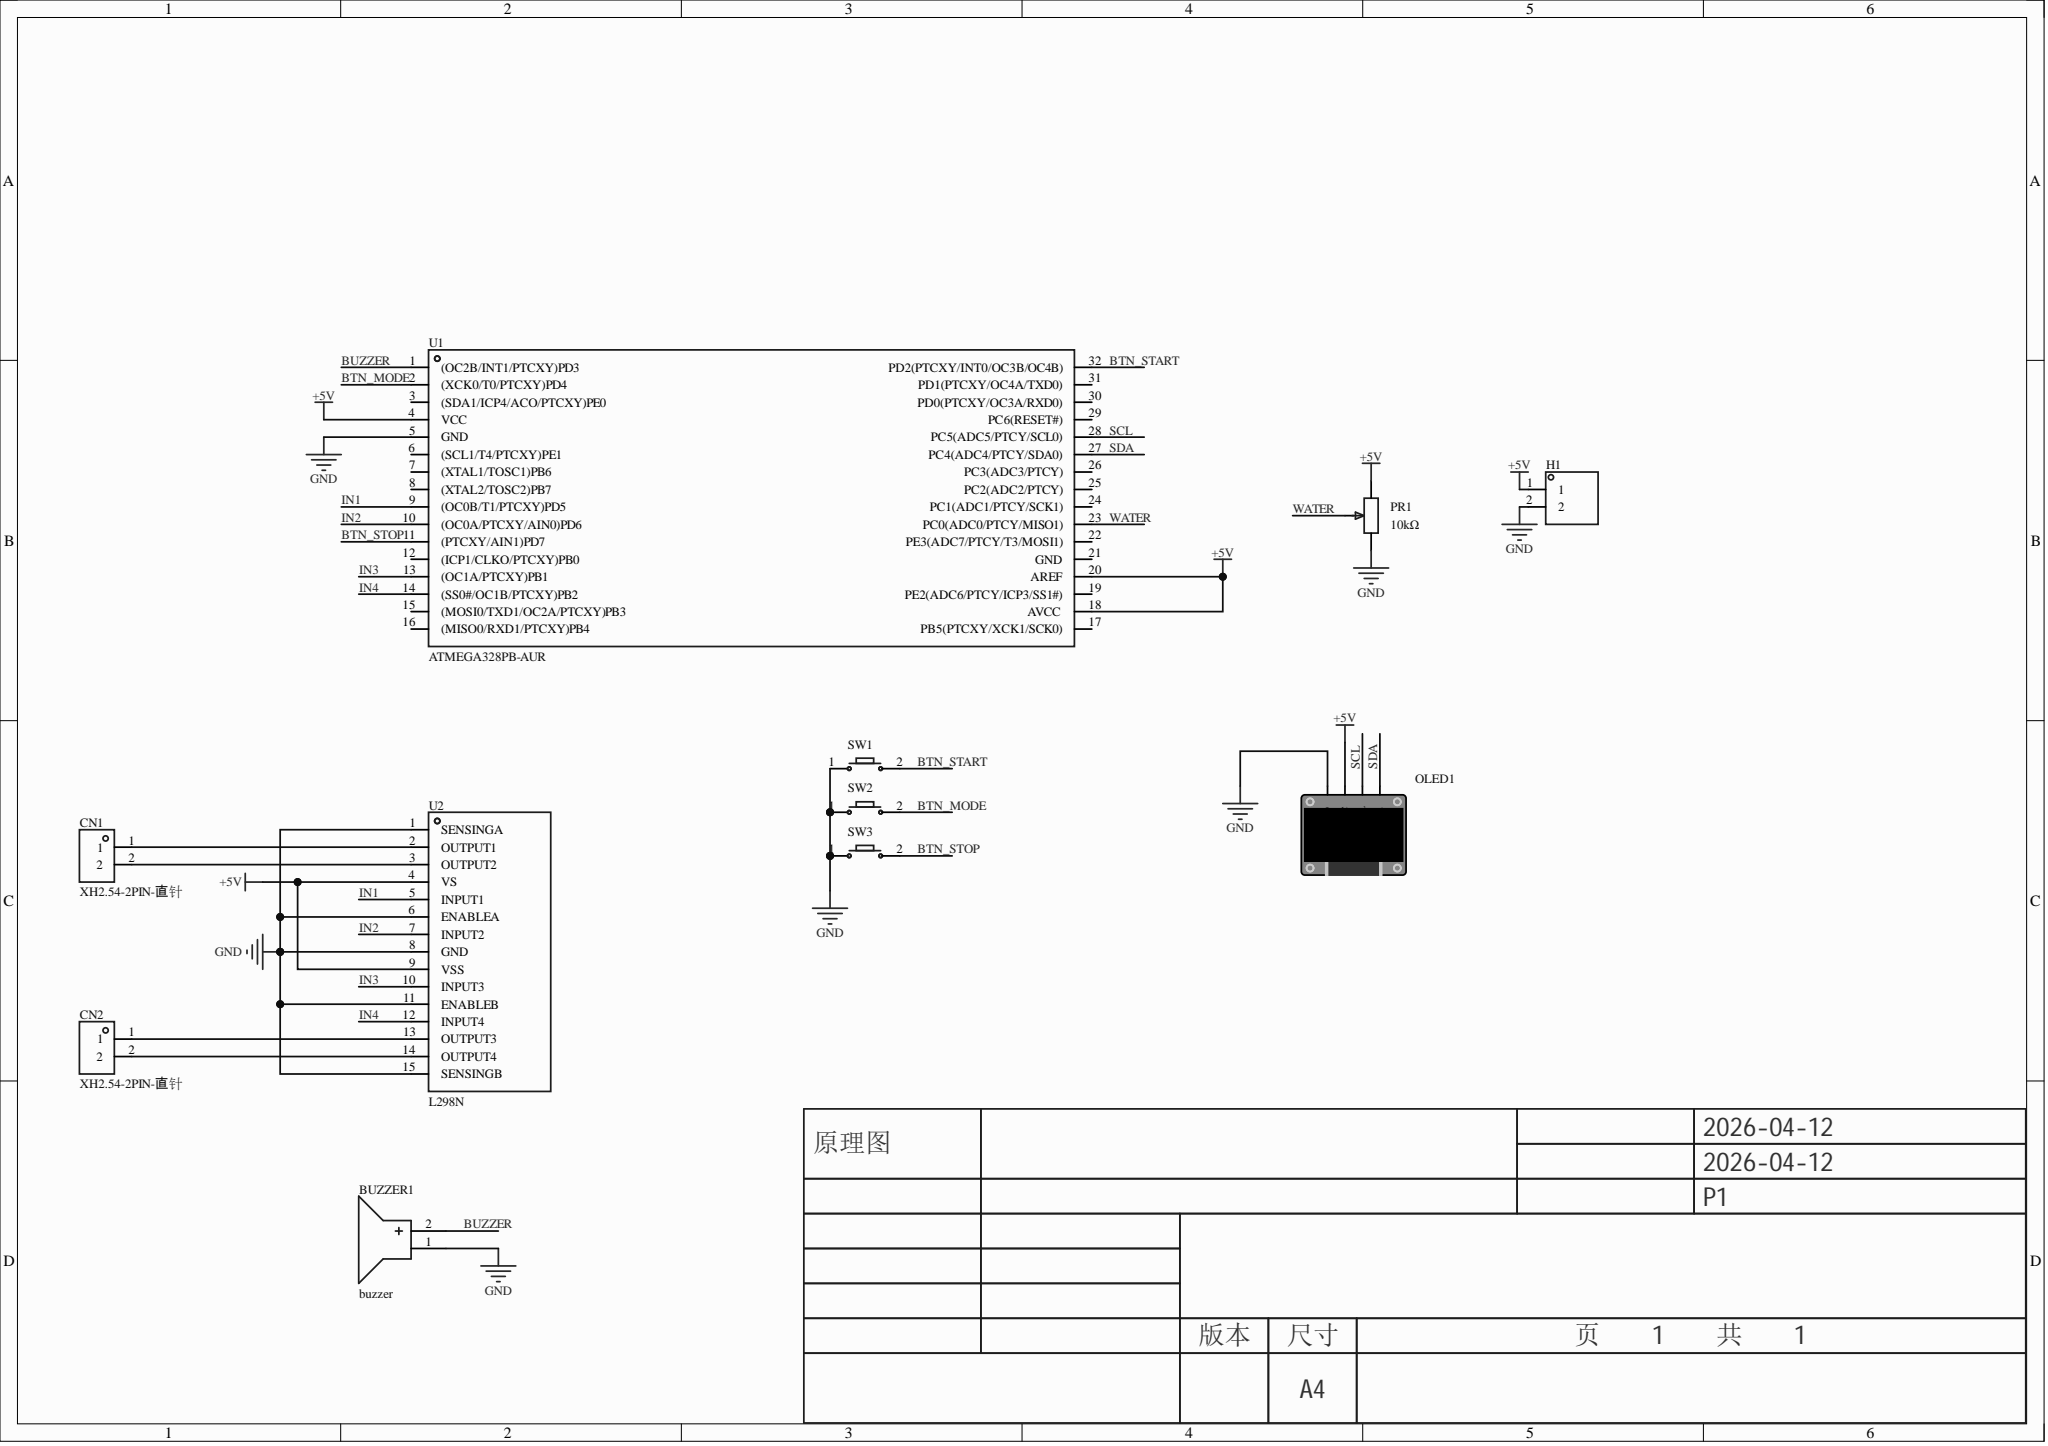Circuit board | Altium Designer | 11 parts | 17 nets
Bill of materials:
Comment,Description,Designator,Footprint,LibRef,Quantity
"buzzer","","BUZZER1","BUZ-TH_BD12.0-P6.00-D0.9-RD","buzzer","1"
"XH2.54-2PIN-直针","","CN1, CN2","CONN-TH_XH2.54-2P","XH2.54-2PIN-直针","2"
"","","H1","HDR-TH_2P-P2.54-V-M-1","HDR-M_2.54_1x2P","1"
"","","OLED1","0.96OLED_4P","0.96OLED模块_4P","1"
"10kΩ","","PR1","R_3296","R_3296","1"
"","","SW1, SW2, SW3","Key_SMD_3x4x2","Key_SMD_3x4x2","3"
"ATMEGA328PB-AUR","","U1","TQFP-32_L7.0-W7.0-P0.80-LS9.0-BL","ATMEGA328PB-AUR","1"
"L298N","","U2","MULTIWATT-15_L19.6-W5.0-P1.27-L","L298N_C504386","1"
Netlist (Protel format):
[
BUZZER1
BUZ-TH_BD12.0-P6.00-D0.9-RD
buzzer



]
[
CN1
CONN-TH_XH2.54-2P
XH2.54-2PIN-直针



]
[
CN2
CONN-TH_XH2.54-2P
XH2.54-2PIN-直针



]
[
H1
HDR-TH_2P-P2.54-V-M-1




]
[
OLED1
0.96OLED_4P




]
[
PR1
R_3296
10kΩ



]
[
SW1
Key_SMD_3x4x2




]
[
SW2
Key_SMD_3x4x2




]
[
SW3
Key_SMD_3x4x2




]
[
U1
TQFP-32_L7.0-W7.0-P0.80-LS9.0-BL
ATMEGA328PB-AUR



]
[
U2
MULTIWATT-15_L19.6-W5.0-P1.27-L
L298N



]
(
WATER
PR1-2
U1-23
)
(
SDA
OLED1-4
U1-27
)
(
SCL
OLED1-3
U1-28
)
(
NetCN2_2
CN2-2
U2-14
)
(
NetCN2_1
CN2-1
U2-13
)
(
NetCN1_2
CN1-2
U2-3
)
(
NetCN1_1
CN1-1
U2-2
)
(
IN4
U1-14
U2-12
)
(
IN3
U1-13
U2-10
)
(
IN2
U1-10
U2-7
)
(
IN1
U1-9
U2-5
)
(
GND
BUZZER1-1
H1-2
OLED1-1
PR1-3
SW1-1
SW2-1
SW3-1
U1-5
U2-1
U2-6
U2-8
U2-11
U2-15
)
(
BUZZER
BUZZER1-2
U1-1
)
(
BTN_STOP
SW3-2
U1-11
)
(
BTN_START
SW1-2
U1-32
)
(
BTN_MODE
SW2-2
U1-2
)
(
+5V
H1-1
OLED1-2
PR1-1
U1-4
U1-18
U1-20
U2-4
U2-9
)